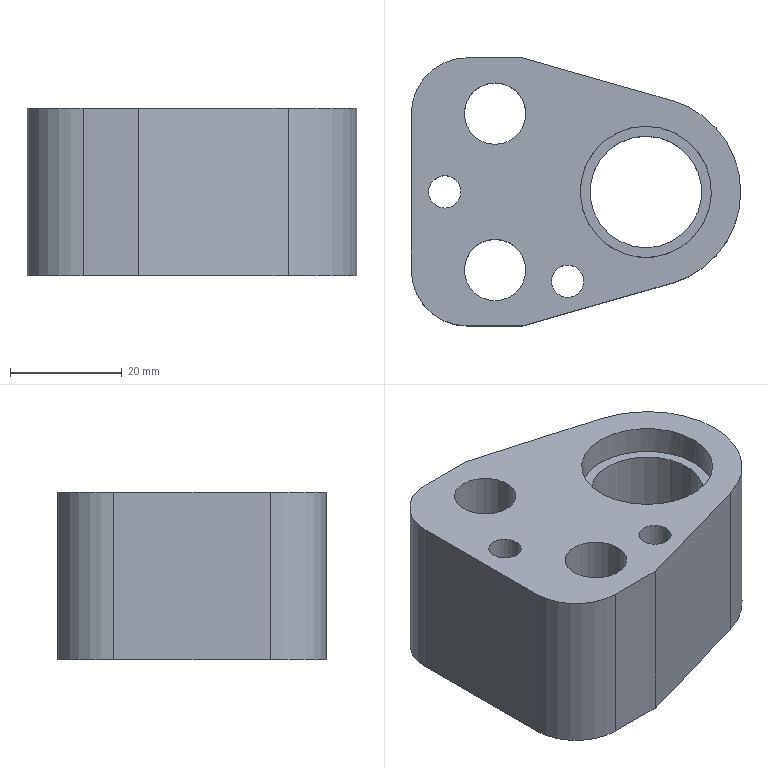Part | NX | features solid 2 | 1 solid | 25 faces | box 59 x 48 x 30 mm | volume 47279 mm3 | cylinder 13 | plane 12 | commonest cylinder face diameters 20 x3 5.8 x2 8 x2 11 x2 17 x2 23.5 x1
STEP:
#1=CARTESIAN_POINT('',(-406.,0.,201.));
#2=VERTEX_POINT('',#1);
#3=CARTESIAN_POINT('',(-379.31,7.66,201.));
#4=VERTEX_POINT('',#3);
#5=CARTESIAN_POINT('',(-386.776,5.517,201.));
#6=DIRECTION('',(0.9612,0.2759,0.));
#7=VECTOR('',#6,1000.);
#8=LINE('',#5,#7);
#9=EDGE_CURVE('',#2,#4,#8,.T.);
#10=ORIENTED_EDGE('',*,*,#9,.T.);
#11=CARTESIAN_POINT('',(-379.31,40.34,201.));
#12=VERTEX_POINT('',#11);
#13=CARTESIAN_POINT('',(-384.,24.,201.));
#14=DIRECTION('',(0.,0.,-1.));
#15=DIRECTION('',(0.,1.,0.));
#16=AXIS2_PLACEMENT_3D('',#13,#14,#15);
#17=CIRCLE('',#16,17.);
#18=EDGE_CURVE('',#12,#4,#17,.T.);
#19=ORIENTED_EDGE('',*,*,#18,.F.);
#20=CARTESIAN_POINT('',(-406.,48.,201.));
#21=VERTEX_POINT('',#20);
#22=CARTESIAN_POINT('',(-386.776,42.483,201.));
#23=DIRECTION('',(-0.9612,0.2759,0.));
#24=VECTOR('',#23,1000.);
#25=LINE('',#22,#24);
#26=EDGE_CURVE('',#12,#21,#25,.T.);
#27=ORIENTED_EDGE('',*,*,#26,.T.);
#28=CARTESIAN_POINT('',(-416.,48.,201.));
#29=VERTEX_POINT('',#28);
#30=CARTESIAN_POINT('',(-392.655,48.,201.));
#31=DIRECTION('',(1.,0.,0.));
#32=VECTOR('',#31,1000.);
#33=LINE('',#30,#32);
#34=EDGE_CURVE('',#29,#21,#33,.T.);
#35=ORIENTED_EDGE('',*,*,#34,.F.);
#36=CARTESIAN_POINT('',(-426.,38.,201.));
#37=VERTEX_POINT('',#36);
#38=CARTESIAN_POINT('',(-416.,38.,201.));
#39=DIRECTION('',(0.,0.,1.));
#40=DIRECTION('',(0.,-1.,0.));
#41=AXIS2_PLACEMENT_3D('',#38,#39,#40);
#42=CIRCLE('',#41,10.);
#43=EDGE_CURVE('',#29,#37,#42,.T.);
#44=ORIENTED_EDGE('',*,*,#43,.T.);
#45=CARTESIAN_POINT('',(-426.,10.,201.));
#46=VERTEX_POINT('',#45);
#47=CARTESIAN_POINT('',(-426.,24.,201.));
#48=DIRECTION('',(0.,1.,0.));
#49=VECTOR('',#48,1000.);
#50=LINE('',#47,#49);
#51=EDGE_CURVE('',#46,#37,#50,.T.);
#52=ORIENTED_EDGE('',*,*,#51,.F.);
#53=CARTESIAN_POINT('',(-416.,0.,201.));
#54=VERTEX_POINT('',#53);
#55=CARTESIAN_POINT('',(-416.,10.,201.));
#56=DIRECTION('',(0.,0.,1.));
#57=DIRECTION('',(0.,-1.,0.));
#58=AXIS2_PLACEMENT_3D('',#55,#56,#57);
#59=CIRCLE('',#58,10.);
#60=EDGE_CURVE('',#46,#54,#59,.T.);
#61=ORIENTED_EDGE('',*,*,#60,.T.);
#62=CARTESIAN_POINT('',(-392.655,0.,201.));
#63=DIRECTION('',(-1.,0.,0.));
#64=VECTOR('',#63,1000.);
#65=LINE('',#62,#64);
#66=EDGE_CURVE('',#2,#54,#65,.T.);
#67=ORIENTED_EDGE('',*,*,#66,.F.);
#68=EDGE_LOOP('',(#10,#19,#27,#35,#44,#52,#61,#67));
#69=FACE_BOUND('',#68,.T.);
#70=CARTESIAN_POINT('',(-420.,26.9,201.));
#71=VERTEX_POINT('',#70);
#72=CARTESIAN_POINT('',(-420.,24.,201.));
#73=DIRECTION('',(0.,0.,-1.));
#74=DIRECTION('',(0.,1.,0.));
#75=AXIS2_PLACEMENT_3D('',#72,#73,#74);
#76=CIRCLE('',#75,2.9);
#77=EDGE_CURVE('',#71,#71,#76,.T.);
#78=ORIENTED_EDGE('',*,*,#77,.T.);
#79=EDGE_LOOP('',(#78));
#80=FACE_BOUND('',#79,.T.);
#81=CARTESIAN_POINT('',(-398.,10.9,201.));
#82=VERTEX_POINT('',#81);
#83=CARTESIAN_POINT('',(-398.,8.,201.));
#84=DIRECTION('',(0.,0.,-1.));
#85=DIRECTION('',(0.,1.,0.));
#86=AXIS2_PLACEMENT_3D('',#83,#84,#85);
#87=CIRCLE('',#86,2.9);
#88=EDGE_CURVE('',#82,#82,#87,.T.);
#89=ORIENTED_EDGE('',*,*,#88,.T.);
#90=EDGE_LOOP('',(#89));
#91=FACE_BOUND('',#90,.T.);
#92=CARTESIAN_POINT('',(-411.,15.5,201.));
#93=VERTEX_POINT('',#92);
#94=CARTESIAN_POINT('',(-411.,10.,201.));
#95=DIRECTION('',(0.,0.,-1.));
#96=DIRECTION('',(0.,1.,0.));
#97=AXIS2_PLACEMENT_3D('',#94,#95,#96);
#98=CIRCLE('',#97,5.5);
#99=EDGE_CURVE('',#93,#93,#98,.T.);
#100=ORIENTED_EDGE('',*,*,#99,.T.);
#101=EDGE_LOOP('',(#100));
#102=FACE_BOUND('',#101,.T.);
#103=CARTESIAN_POINT('',(-411.,43.5,201.));
#104=VERTEX_POINT('',#103);
#105=CARTESIAN_POINT('',(-411.,38.,201.));
#106=DIRECTION('',(0.,0.,-1.));
#107=DIRECTION('',(0.,1.,0.));
#108=AXIS2_PLACEMENT_3D('',#105,#106,#107);
#109=CIRCLE('',#108,5.5);
#110=EDGE_CURVE('',#104,#104,#109,.T.);
#111=ORIENTED_EDGE('',*,*,#110,.T.);
#112=EDGE_LOOP('',(#111));
#113=FACE_BOUND('',#112,.T.);
#114=CARTESIAN_POINT('',(-384.,35.75,201.));
#115=VERTEX_POINT('',#114);
#116=CARTESIAN_POINT('',(-384.,24.,201.));
#117=DIRECTION('',(0.,0.,-1.));
#118=DIRECTION('',(0.,1.,0.));
#119=AXIS2_PLACEMENT_3D('',#116,#117,#118);
#120=CIRCLE('',#119,11.75);
#121=EDGE_CURVE('',#115,#115,#120,.T.);
#122=ORIENTED_EDGE('',*,*,#121,.T.);
#123=EDGE_LOOP('',(#122));
#124=FACE_BOUND('',#123,.T.);
#125=CARTESIAN_POINT('',(-392.655,24.,201.));
#126=DIRECTION('',(0.,0.,1.));
#127=DIRECTION('',(0.,-1.,0.));
#128=AXIS2_PLACEMENT_3D('',#125,#126,#127);
#129=PLANE('',#128);
#130=ADVANCED_FACE('',(#69,#80,#91,#102,#113,#124),#129,.T.);
#131=CARTESIAN_POINT('',(-406.,48.,171.));
#132=VERTEX_POINT('',#131);
#133=CARTESIAN_POINT('',(-406.,48.,171.));
#134=DIRECTION('',(0.,0.,1.));
#135=VECTOR('',#134,1000.);
#136=LINE('',#133,#135);
#137=EDGE_CURVE('',#132,#21,#136,.T.);
#138=ORIENTED_EDGE('',*,*,#137,.F.);
#139=CARTESIAN_POINT('',(-416.,48.,171.));
#140=VERTEX_POINT('',#139);
#141=CARTESIAN_POINT('',(-392.655,48.,171.));
#142=DIRECTION('',(-1.,0.,0.));
#143=VECTOR('',#142,1000.);
#144=LINE('',#141,#143);
#145=EDGE_CURVE('',#132,#140,#144,.T.);
#146=ORIENTED_EDGE('',*,*,#145,.T.);
#147=CARTESIAN_POINT('',(-416.,48.,171.));
#148=DIRECTION('',(0.,0.,1.));
#149=VECTOR('',#148,1000.);
#150=LINE('',#147,#149);
#151=EDGE_CURVE('',#140,#29,#150,.T.);
#152=ORIENTED_EDGE('',*,*,#151,.T.);
#153=ORIENTED_EDGE('',*,*,#34,.T.);
#154=EDGE_LOOP('',(#138,#146,#152,#153));
#155=FACE_BOUND('',#154,.T.);
#156=CARTESIAN_POINT('',(-392.655,48.,171.));
#157=DIRECTION('',(0.,1.,0.));
#158=DIRECTION('',(0.,0.,1.));
#159=AXIS2_PLACEMENT_3D('',#156,#157,#158);
#160=PLANE('',#159);
#161=ADVANCED_FACE('',(#155),#160,.T.);
#162=CARTESIAN_POINT('',(-379.31,7.66,171.));
#163=VERTEX_POINT('',#162);
#164=CARTESIAN_POINT('',(-406.,0.,171.));
#165=VERTEX_POINT('',#164);
#166=CARTESIAN_POINT('',(-386.776,5.517,171.));
#167=DIRECTION('',(-0.9612,-0.2759,0.));
#168=VECTOR('',#167,1000.);
#169=LINE('',#166,#168);
#170=EDGE_CURVE('',#163,#165,#169,.T.);
#171=ORIENTED_EDGE('',*,*,#170,.T.);
#172=CARTESIAN_POINT('',(-416.,0.,171.));
#173=VERTEX_POINT('',#172);
#174=CARTESIAN_POINT('',(-392.655,0.,171.));
#175=DIRECTION('',(1.,0.,0.));
#176=VECTOR('',#175,1000.);
#177=LINE('',#174,#176);
#178=EDGE_CURVE('',#173,#165,#177,.T.);
#179=ORIENTED_EDGE('',*,*,#178,.F.);
#180=CARTESIAN_POINT('',(-426.,10.,171.));
#181=VERTEX_POINT('',#180);
#182=CARTESIAN_POINT('',(-416.,10.,171.));
#183=DIRECTION('',(0.,0.,-1.));
#184=DIRECTION('',(0.,1.,0.));
#185=AXIS2_PLACEMENT_3D('',#182,#183,#184);
#186=CIRCLE('',#185,10.);
#187=EDGE_CURVE('',#173,#181,#186,.T.);
#188=ORIENTED_EDGE('',*,*,#187,.T.);
#189=CARTESIAN_POINT('',(-426.,38.,171.));
#190=VERTEX_POINT('',#189);
#191=CARTESIAN_POINT('',(-426.,24.,171.));
#192=DIRECTION('',(0.,-1.,0.));
#193=VECTOR('',#192,1000.);
#194=LINE('',#191,#193);
#195=EDGE_CURVE('',#190,#181,#194,.T.);
#196=ORIENTED_EDGE('',*,*,#195,.F.);
#197=CARTESIAN_POINT('',(-416.,38.,171.));
#198=DIRECTION('',(0.,0.,-1.));
#199=DIRECTION('',(0.,1.,0.));
#200=AXIS2_PLACEMENT_3D('',#197,#198,#199);
#201=CIRCLE('',#200,10.);
#202=EDGE_CURVE('',#190,#140,#201,.T.);
#203=ORIENTED_EDGE('',*,*,#202,.T.);
#204=ORIENTED_EDGE('',*,*,#145,.F.);
#205=CARTESIAN_POINT('',(-379.31,40.34,171.));
#206=VERTEX_POINT('',#205);
#207=CARTESIAN_POINT('',(-386.776,42.483,171.));
#208=DIRECTION('',(0.9612,-0.2759,0.));
#209=VECTOR('',#208,1000.);
#210=LINE('',#207,#209);
#211=EDGE_CURVE('',#132,#206,#210,.T.);
#212=ORIENTED_EDGE('',*,*,#211,.T.);
#213=CARTESIAN_POINT('',(-384.,24.,171.));
#214=DIRECTION('',(0.,0.,1.));
#215=DIRECTION('',(0.,-1.,0.));
#216=AXIS2_PLACEMENT_3D('',#213,#214,#215);
#217=CIRCLE('',#216,17.);
#218=EDGE_CURVE('',#163,#206,#217,.T.);
#219=ORIENTED_EDGE('',*,*,#218,.F.);
#220=EDGE_LOOP('',(#171,#179,#188,#196,#203,#204,#212,#219));
#221=FACE_BOUND('',#220,.T.);
#222=CARTESIAN_POINT('',(-420.,20.,171.));
#223=VERTEX_POINT('',#222);
#224=CARTESIAN_POINT('',(-420.,24.,171.));
#225=DIRECTION('',(0.,0.,1.));
#226=DIRECTION('',(0.,-1.,0.));
#227=AXIS2_PLACEMENT_3D('',#224,#225,#226);
#228=CIRCLE('',#227,4.);
#229=EDGE_CURVE('',#223,#223,#228,.T.);
#230=ORIENTED_EDGE('',*,*,#229,.T.);
#231=EDGE_LOOP('',(#230));
#232=FACE_BOUND('',#231,.T.);
#233=CARTESIAN_POINT('',(-398.,4.,171.));
#234=VERTEX_POINT('',#233);
#235=CARTESIAN_POINT('',(-398.,8.,171.));
#236=DIRECTION('',(0.,0.,1.));
#237=DIRECTION('',(0.,-1.,0.));
#238=AXIS2_PLACEMENT_3D('',#235,#236,#237);
#239=CIRCLE('',#238,4.);
#240=EDGE_CURVE('',#234,#234,#239,.T.);
#241=ORIENTED_EDGE('',*,*,#240,.T.);
#242=EDGE_LOOP('',(#241));
#243=FACE_BOUND('',#242,.T.);
#244=CARTESIAN_POINT('',(-411.,1.5,171.));
#245=VERTEX_POINT('',#244);
#246=CARTESIAN_POINT('',(-411.,10.,171.));
#247=DIRECTION('',(0.,0.,1.));
#248=DIRECTION('',(0.,-1.,0.));
#249=AXIS2_PLACEMENT_3D('',#246,#247,#248);
#250=CIRCLE('',#249,8.5);
#251=EDGE_CURVE('',#245,#245,#250,.T.);
#252=ORIENTED_EDGE('',*,*,#251,.T.);
#253=EDGE_LOOP('',(#252));
#254=FACE_BOUND('',#253,.T.);
#255=CARTESIAN_POINT('',(-411.,29.5,171.));
#256=VERTEX_POINT('',#255);
#257=CARTESIAN_POINT('',(-411.,38.,171.));
#258=DIRECTION('',(0.,0.,1.));
#259=DIRECTION('',(0.,-1.,0.));
#260=AXIS2_PLACEMENT_3D('',#257,#258,#259);
#261=CIRCLE('',#260,8.5);
#262=EDGE_CURVE('',#256,#256,#261,.T.);
#263=ORIENTED_EDGE('',*,*,#262,.T.);
#264=EDGE_LOOP('',(#263));
#265=FACE_BOUND('',#264,.T.);
#266=CARTESIAN_POINT('',(-384.,14.,171.));
#267=VERTEX_POINT('',#266);
#268=CARTESIAN_POINT('',(-384.,24.,171.));
#269=DIRECTION('',(0.,0.,1.));
#270=DIRECTION('',(0.,-1.,0.));
#271=AXIS2_PLACEMENT_3D('',#268,#269,#270);
#272=CIRCLE('',#271,10.);
#273=EDGE_CURVE('',#267,#267,#272,.T.);
#274=ORIENTED_EDGE('',*,*,#273,.T.);
#275=EDGE_LOOP('',(#274));
#276=FACE_BOUND('',#275,.T.);
#277=CARTESIAN_POINT('',(-392.655,24.,171.));
#278=DIRECTION('',(0.,0.,-1.));
#279=DIRECTION('',(0.,1.,0.));
#280=AXIS2_PLACEMENT_3D('',#277,#278,#279);
#281=PLANE('',#280);
#282=ADVANCED_FACE('',(#221,#232,#243,#254,#265,#276),#281,.T.);
#283=CARTESIAN_POINT('',(-406.,0.,171.));
#284=DIRECTION('',(0.,0.,1.));
#285=VECTOR('',#284,1000.);
#286=LINE('',#283,#285);
#287=EDGE_CURVE('',#165,#2,#286,.T.);
#288=ORIENTED_EDGE('',*,*,#287,.T.);
#289=ORIENTED_EDGE('',*,*,#66,.T.);
#290=CARTESIAN_POINT('',(-416.,0.,171.));
#291=DIRECTION('',(0.,0.,1.));
#292=VECTOR('',#291,1000.);
#293=LINE('',#290,#292);
#294=EDGE_CURVE('',#54,#173,#293,.F.);
#295=ORIENTED_EDGE('',*,*,#294,.T.);
#296=ORIENTED_EDGE('',*,*,#178,.T.);
#297=EDGE_LOOP('',(#288,#289,#295,#296));
#298=FACE_BOUND('',#297,.T.);
#299=CARTESIAN_POINT('',(-392.655,0.,171.));
#300=DIRECTION('',(0.,-1.,0.));
#301=DIRECTION('',(0.,0.,-1.));
#302=AXIS2_PLACEMENT_3D('',#299,#300,#301);
#303=PLANE('',#302);
#304=ADVANCED_FACE('',(#298),#303,.T.);
#305=ORIENTED_EDGE('',*,*,#18,.T.);
#306=CARTESIAN_POINT('',(-379.31,7.66,201.));
#307=DIRECTION('',(0.,0.,-1.));
#308=VECTOR('',#307,1000.);
#309=LINE('',#306,#308);
#310=EDGE_CURVE('',#4,#163,#309,.T.);
#311=ORIENTED_EDGE('',*,*,#310,.T.);
#312=ORIENTED_EDGE('',*,*,#218,.T.);
#313=CARTESIAN_POINT('',(-379.31,40.34,201.));
#314=DIRECTION('',(0.,0.,-1.));
#315=VECTOR('',#314,1000.);
#316=LINE('',#313,#315);
#317=EDGE_CURVE('',#206,#12,#316,.F.);
#318=ORIENTED_EDGE('',*,*,#317,.T.);
#319=EDGE_LOOP('',(#305,#311,#312,#318));
#320=FACE_BOUND('',#319,.T.);
#321=CARTESIAN_POINT('',(-384.,24.,201.));
#322=DIRECTION('',(0.,0.,-1.));
#323=DIRECTION('',(0.,1.,0.));
#324=AXIS2_PLACEMENT_3D('',#321,#322,#323);
#325=CYLINDRICAL_SURFACE('',#324,17.);
#326=ADVANCED_FACE('',(#320),#325,.T.);
#327=ORIENTED_EDGE('',*,*,#195,.T.);
#328=CARTESIAN_POINT('',(-426.,10.,171.));
#329=DIRECTION('',(0.,0.,1.));
#330=VECTOR('',#329,1000.);
#331=LINE('',#328,#330);
#332=EDGE_CURVE('',#181,#46,#331,.T.);
#333=ORIENTED_EDGE('',*,*,#332,.T.);
#334=ORIENTED_EDGE('',*,*,#51,.T.);
#335=CARTESIAN_POINT('',(-426.,38.,171.));
#336=DIRECTION('',(0.,0.,1.));
#337=VECTOR('',#336,1000.);
#338=LINE('',#335,#337);
#339=EDGE_CURVE('',#37,#190,#338,.F.);
#340=ORIENTED_EDGE('',*,*,#339,.T.);
#341=EDGE_LOOP('',(#327,#333,#334,#340));
#342=FACE_BOUND('',#341,.T.);
#343=CARTESIAN_POINT('',(-426.,24.,171.));
#344=DIRECTION('',(-1.,0.,0.));
#345=DIRECTION('',(0.,0.,-1.));
#346=AXIS2_PLACEMENT_3D('',#343,#344,#345);
#347=PLANE('',#346);
#348=ADVANCED_FACE('',(#342),#347,.T.);
#349=CARTESIAN_POINT('',(-384.,34.,196.));
#350=VERTEX_POINT('',#349);
#351=CARTESIAN_POINT('',(-384.,24.,196.));
#352=DIRECTION('',(0.,0.,-1.));
#353=DIRECTION('',(0.,1.,0.));
#354=AXIS2_PLACEMENT_3D('',#351,#352,#353);
#355=CIRCLE('',#354,10.);
#356=EDGE_CURVE('',#350,#350,#355,.T.);
#357=ORIENTED_EDGE('',*,*,#356,.T.);
#358=EDGE_LOOP('',(#357));
#359=FACE_BOUND('',#358,.T.);
#360=CARTESIAN_POINT('',(-384.,12.25,196.));
#361=VERTEX_POINT('',#360);
#362=CARTESIAN_POINT('',(-384.,24.,196.));
#363=DIRECTION('',(0.,0.,1.));
#364=DIRECTION('',(0.,-1.,0.));
#365=AXIS2_PLACEMENT_3D('',#362,#363,#364);
#366=CIRCLE('',#365,11.75);
#367=EDGE_CURVE('',#361,#361,#366,.T.);
#368=ORIENTED_EDGE('',*,*,#367,.T.);
#369=EDGE_LOOP('',(#368));
#370=FACE_BOUND('',#369,.T.);
#371=CARTESIAN_POINT('',(-384.,24.,196.));
#372=DIRECTION('',(0.,0.,-1.));
#373=DIRECTION('',(0.,1.,0.));
#374=AXIS2_PLACEMENT_3D('',#371,#372,#373);
#375=PLANE('',#374);
#376=ADVANCED_FACE('',(#359,#370),#375,.F.);
#377=ORIENTED_EDGE('',*,*,#367,.F.);
#378=EDGE_LOOP('',(#377));
#379=FACE_BOUND('',#378,.T.);
#380=ORIENTED_EDGE('',*,*,#121,.F.);
#381=EDGE_LOOP('',(#380));
#382=FACE_BOUND('',#381,.T.);
#383=CARTESIAN_POINT('',(-384.,24.,201.));
#384=DIRECTION('',(0.,0.,-1.));
#385=DIRECTION('',(0.,1.,0.));
#386=AXIS2_PLACEMENT_3D('',#383,#384,#385);
#387=CYLINDRICAL_SURFACE('',#386,11.75);
#388=ADVANCED_FACE('',(#379,#382),#387,.F.);
#389=ORIENTED_EDGE('',*,*,#273,.F.);
#390=EDGE_LOOP('',(#389));
#391=FACE_BOUND('',#390,.T.);
#392=ORIENTED_EDGE('',*,*,#356,.F.);
#393=EDGE_LOOP('',(#392));
#394=FACE_BOUND('',#393,.T.);
#395=CARTESIAN_POINT('',(-384.,24.,196.));
#396=DIRECTION('',(0.,0.,-1.));
#397=DIRECTION('',(0.,1.,0.));
#398=AXIS2_PLACEMENT_3D('',#395,#396,#397);
#399=CYLINDRICAL_SURFACE('',#398,10.);
#400=ADVANCED_FACE('',(#391,#394),#399,.F.);
#401=CARTESIAN_POINT('',(-411.,32.5,183.));
#402=VERTEX_POINT('',#401);
#403=CARTESIAN_POINT('',(-411.,38.,183.));
#404=DIRECTION('',(0.,0.,1.));
#405=DIRECTION('',(0.,-1.,0.));
#406=AXIS2_PLACEMENT_3D('',#403,#404,#405);
#407=CIRCLE('',#406,5.5);
#408=EDGE_CURVE('',#402,#402,#407,.F.);
#409=ORIENTED_EDGE('',*,*,#408,.T.);
#410=EDGE_LOOP('',(#409));
#411=FACE_BOUND('',#410,.T.);
#412=ORIENTED_EDGE('',*,*,#110,.F.);
#413=EDGE_LOOP('',(#412));
#414=FACE_BOUND('',#413,.T.);
#415=CARTESIAN_POINT('',(-411.,38.,201.));
#416=DIRECTION('',(0.,0.,-1.));
#417=DIRECTION('',(0.,1.,0.));
#418=AXIS2_PLACEMENT_3D('',#415,#416,#417);
#419=CYLINDRICAL_SURFACE('',#418,5.5);
#420=ADVANCED_FACE('',(#411,#414),#419,.F.);
#421=CARTESIAN_POINT('',(-411.,46.5,183.));
#422=VERTEX_POINT('',#421);
#423=CARTESIAN_POINT('',(-411.,38.,183.));
#424=DIRECTION('',(0.,0.,-1.));
#425=DIRECTION('',(0.,1.,0.));
#426=AXIS2_PLACEMENT_3D('',#423,#424,#425);
#427=CIRCLE('',#426,8.5);
#428=EDGE_CURVE('',#422,#422,#427,.T.);
#429=ORIENTED_EDGE('',*,*,#428,.T.);
#430=EDGE_LOOP('',(#429));
#431=FACE_BOUND('',#430,.T.);
#432=ORIENTED_EDGE('',*,*,#408,.F.);
#433=EDGE_LOOP('',(#432));
#434=FACE_BOUND('',#433,.T.);
#435=CARTESIAN_POINT('',(-411.,38.,183.));
#436=DIRECTION('',(0.,0.,1.));
#437=DIRECTION('',(0.,-1.,0.));
#438=AXIS2_PLACEMENT_3D('',#435,#436,#437);
#439=PLANE('',#438);
#440=ADVANCED_FACE('',(#431,#434),#439,.F.);
#441=ORIENTED_EDGE('',*,*,#262,.F.);
#442=EDGE_LOOP('',(#441));
#443=FACE_BOUND('',#442,.T.);
#444=ORIENTED_EDGE('',*,*,#428,.F.);
#445=EDGE_LOOP('',(#444));
#446=FACE_BOUND('',#445,.T.);
#447=CARTESIAN_POINT('',(-411.,38.,183.));
#448=DIRECTION('',(0.,0.,-1.));
#449=DIRECTION('',(0.,1.,0.));
#450=AXIS2_PLACEMENT_3D('',#447,#448,#449);
#451=CYLINDRICAL_SURFACE('',#450,8.5);
#452=ADVANCED_FACE('',(#443,#446),#451,.F.);
#453=CARTESIAN_POINT('',(-411.,4.5,183.));
#454=VERTEX_POINT('',#453);
#455=CARTESIAN_POINT('',(-411.,10.,183.));
#456=DIRECTION('',(0.,0.,1.));
#457=DIRECTION('',(0.,-1.,0.));
#458=AXIS2_PLACEMENT_3D('',#455,#456,#457);
#459=CIRCLE('',#458,5.5);
#460=EDGE_CURVE('',#454,#454,#459,.F.);
#461=ORIENTED_EDGE('',*,*,#460,.T.);
#462=EDGE_LOOP('',(#461));
#463=FACE_BOUND('',#462,.T.);
#464=ORIENTED_EDGE('',*,*,#99,.F.);
#465=EDGE_LOOP('',(#464));
#466=FACE_BOUND('',#465,.T.);
#467=CARTESIAN_POINT('',(-411.,10.,201.));
#468=DIRECTION('',(0.,0.,-1.));
#469=DIRECTION('',(0.,1.,0.));
#470=AXIS2_PLACEMENT_3D('',#467,#468,#469);
#471=CYLINDRICAL_SURFACE('',#470,5.5);
#472=ADVANCED_FACE('',(#463,#466),#471,.F.);
#473=CARTESIAN_POINT('',(-411.,18.5,183.));
#474=VERTEX_POINT('',#473);
#475=CARTESIAN_POINT('',(-411.,10.,183.));
#476=DIRECTION('',(0.,0.,-1.));
#477=DIRECTION('',(0.,1.,0.));
#478=AXIS2_PLACEMENT_3D('',#475,#476,#477);
#479=CIRCLE('',#478,8.5);
#480=EDGE_CURVE('',#474,#474,#479,.T.);
#481=ORIENTED_EDGE('',*,*,#480,.T.);
#482=EDGE_LOOP('',(#481));
#483=FACE_BOUND('',#482,.T.);
#484=ORIENTED_EDGE('',*,*,#460,.F.);
#485=EDGE_LOOP('',(#484));
#486=FACE_BOUND('',#485,.T.);
#487=CARTESIAN_POINT('',(-411.,10.,183.));
#488=DIRECTION('',(0.,0.,1.));
#489=DIRECTION('',(0.,-1.,0.));
#490=AXIS2_PLACEMENT_3D('',#487,#488,#489);
#491=PLANE('',#490);
#492=ADVANCED_FACE('',(#483,#486),#491,.F.);
#493=ORIENTED_EDGE('',*,*,#251,.F.);
#494=EDGE_LOOP('',(#493));
#495=FACE_BOUND('',#494,.T.);
#496=ORIENTED_EDGE('',*,*,#480,.F.);
#497=EDGE_LOOP('',(#496));
#498=FACE_BOUND('',#497,.T.);
#499=CARTESIAN_POINT('',(-411.,10.,183.));
#500=DIRECTION('',(0.,0.,-1.));
#501=DIRECTION('',(0.,1.,0.));
#502=AXIS2_PLACEMENT_3D('',#499,#500,#501);
#503=CYLINDRICAL_SURFACE('',#502,8.5);
#504=ADVANCED_FACE('',(#495,#498),#503,.F.);
#505=CARTESIAN_POINT('',(-398.,5.1,191.));
#506=VERTEX_POINT('',#505);
#507=CARTESIAN_POINT('',(-398.,8.,191.));
#508=DIRECTION('',(0.,0.,1.));
#509=DIRECTION('',(0.,-1.,0.));
#510=AXIS2_PLACEMENT_3D('',#507,#508,#509);
#511=CIRCLE('',#510,2.9);
#512=EDGE_CURVE('',#506,#506,#511,.F.);
#513=ORIENTED_EDGE('',*,*,#512,.T.);
#514=EDGE_LOOP('',(#513));
#515=FACE_BOUND('',#514,.T.);
#516=ORIENTED_EDGE('',*,*,#88,.F.);
#517=EDGE_LOOP('',(#516));
#518=FACE_BOUND('',#517,.T.);
#519=CARTESIAN_POINT('',(-398.,8.,201.));
#520=DIRECTION('',(0.,0.,-1.));
#521=DIRECTION('',(0.,1.,0.));
#522=AXIS2_PLACEMENT_3D('',#519,#520,#521);
#523=CYLINDRICAL_SURFACE('',#522,2.9);
#524=ADVANCED_FACE('',(#515,#518),#523,.F.);
#525=CARTESIAN_POINT('',(-398.,12.,191.));
#526=VERTEX_POINT('',#525);
#527=CARTESIAN_POINT('',(-398.,8.,191.));
#528=DIRECTION('',(0.,0.,-1.));
#529=DIRECTION('',(0.,1.,0.));
#530=AXIS2_PLACEMENT_3D('',#527,#528,#529);
#531=CIRCLE('',#530,4.);
#532=EDGE_CURVE('',#526,#526,#531,.T.);
#533=ORIENTED_EDGE('',*,*,#532,.T.);
#534=EDGE_LOOP('',(#533));
#535=FACE_BOUND('',#534,.T.);
#536=ORIENTED_EDGE('',*,*,#512,.F.);
#537=EDGE_LOOP('',(#536));
#538=FACE_BOUND('',#537,.T.);
#539=CARTESIAN_POINT('',(-398.,8.,191.));
#540=DIRECTION('',(0.,0.,1.));
#541=DIRECTION('',(0.,-1.,0.));
#542=AXIS2_PLACEMENT_3D('',#539,#540,#541);
#543=PLANE('',#542);
#544=ADVANCED_FACE('',(#535,#538),#543,.F.);
#545=ORIENTED_EDGE('',*,*,#240,.F.);
#546=EDGE_LOOP('',(#545));
#547=FACE_BOUND('',#546,.T.);
#548=ORIENTED_EDGE('',*,*,#532,.F.);
#549=EDGE_LOOP('',(#548));
#550=FACE_BOUND('',#549,.T.);
#551=CARTESIAN_POINT('',(-398.,8.,191.));
#552=DIRECTION('',(0.,0.,-1.));
#553=DIRECTION('',(0.,1.,0.));
#554=AXIS2_PLACEMENT_3D('',#551,#552,#553);
#555=CYLINDRICAL_SURFACE('',#554,4.);
#556=ADVANCED_FACE('',(#547,#550),#555,.F.);
#557=CARTESIAN_POINT('',(-420.,21.1,191.));
#558=VERTEX_POINT('',#557);
#559=CARTESIAN_POINT('',(-420.,24.,191.));
#560=DIRECTION('',(0.,0.,1.));
#561=DIRECTION('',(0.,-1.,0.));
#562=AXIS2_PLACEMENT_3D('',#559,#560,#561);
#563=CIRCLE('',#562,2.9);
#564=EDGE_CURVE('',#558,#558,#563,.F.);
#565=ORIENTED_EDGE('',*,*,#564,.T.);
#566=EDGE_LOOP('',(#565));
#567=FACE_BOUND('',#566,.T.);
#568=ORIENTED_EDGE('',*,*,#77,.F.);
#569=EDGE_LOOP('',(#568));
#570=FACE_BOUND('',#569,.T.);
#571=CARTESIAN_POINT('',(-420.,24.,201.));
#572=DIRECTION('',(0.,0.,-1.));
#573=DIRECTION('',(0.,1.,0.));
#574=AXIS2_PLACEMENT_3D('',#571,#572,#573);
#575=CYLINDRICAL_SURFACE('',#574,2.9);
#576=ADVANCED_FACE('',(#567,#570),#575,.F.);
#577=CARTESIAN_POINT('',(-420.,28.,191.));
#578=VERTEX_POINT('',#577);
#579=CARTESIAN_POINT('',(-420.,24.,191.));
#580=DIRECTION('',(0.,0.,-1.));
#581=DIRECTION('',(0.,1.,0.));
#582=AXIS2_PLACEMENT_3D('',#579,#580,#581);
#583=CIRCLE('',#582,4.);
#584=EDGE_CURVE('',#578,#578,#583,.T.);
#585=ORIENTED_EDGE('',*,*,#584,.T.);
#586=EDGE_LOOP('',(#585));
#587=FACE_BOUND('',#586,.T.);
#588=ORIENTED_EDGE('',*,*,#564,.F.);
#589=EDGE_LOOP('',(#588));
#590=FACE_BOUND('',#589,.T.);
#591=CARTESIAN_POINT('',(-420.,24.,191.));
#592=DIRECTION('',(0.,0.,1.));
#593=DIRECTION('',(0.,-1.,0.));
#594=AXIS2_PLACEMENT_3D('',#591,#592,#593);
#595=PLANE('',#594);
#596=ADVANCED_FACE('',(#587,#590),#595,.F.);
#597=ORIENTED_EDGE('',*,*,#229,.F.);
#598=EDGE_LOOP('',(#597));
#599=FACE_BOUND('',#598,.T.);
#600=ORIENTED_EDGE('',*,*,#584,.F.);
#601=EDGE_LOOP('',(#600));
#602=FACE_BOUND('',#601,.T.);
#603=CARTESIAN_POINT('',(-420.,24.,191.));
#604=DIRECTION('',(0.,0.,-1.));
#605=DIRECTION('',(0.,1.,0.));
#606=AXIS2_PLACEMENT_3D('',#603,#604,#605);
#607=CYLINDRICAL_SURFACE('',#606,4.);
#608=ADVANCED_FACE('',(#599,#602),#607,.F.);
#609=ORIENTED_EDGE('',*,*,#187,.F.);
#610=ORIENTED_EDGE('',*,*,#294,.F.);
#611=ORIENTED_EDGE('',*,*,#60,.F.);
#612=ORIENTED_EDGE('',*,*,#332,.F.);
#613=EDGE_LOOP('',(#609,#610,#611,#612));
#614=FACE_BOUND('',#613,.T.);
#615=CARTESIAN_POINT('',(-416.,10.,171.));
#616=DIRECTION('',(0.,0.,1.));
#617=DIRECTION('',(0.,-1.,0.));
#618=AXIS2_PLACEMENT_3D('',#615,#616,#617);
#619=CYLINDRICAL_SURFACE('',#618,10.);
#620=ADVANCED_FACE('',(#614),#619,.T.);
#621=ORIENTED_EDGE('',*,*,#202,.F.);
#622=ORIENTED_EDGE('',*,*,#339,.F.);
#623=ORIENTED_EDGE('',*,*,#43,.F.);
#624=ORIENTED_EDGE('',*,*,#151,.F.);
#625=EDGE_LOOP('',(#621,#622,#623,#624));
#626=FACE_BOUND('',#625,.T.);
#627=CARTESIAN_POINT('',(-416.,38.,171.));
#628=DIRECTION('',(0.,0.,1.));
#629=DIRECTION('',(0.,-1.,0.));
#630=AXIS2_PLACEMENT_3D('',#627,#628,#629);
#631=CYLINDRICAL_SURFACE('',#630,10.);
#632=ADVANCED_FACE('',(#626),#631,.T.);
#633=ORIENTED_EDGE('',*,*,#317,.F.);
#634=ORIENTED_EDGE('',*,*,#211,.F.);
#635=ORIENTED_EDGE('',*,*,#137,.T.);
#636=ORIENTED_EDGE('',*,*,#26,.F.);
#637=EDGE_LOOP('',(#633,#634,#635,#636));
#638=FACE_BOUND('',#637,.T.);
#639=CARTESIAN_POINT('',(-386.776,42.483,171.));
#640=DIRECTION('',(-0.2759,-0.9612,0.));
#641=DIRECTION('',(0.,0.,-1.));
#642=AXIS2_PLACEMENT_3D('',#639,#640,#641);
#643=PLANE('',#642);
#644=ADVANCED_FACE('',(#638),#643,.F.);
#645=ORIENTED_EDGE('',*,*,#310,.F.);
#646=ORIENTED_EDGE('',*,*,#9,.F.);
#647=ORIENTED_EDGE('',*,*,#287,.F.);
#648=ORIENTED_EDGE('',*,*,#170,.F.);
#649=EDGE_LOOP('',(#645,#646,#647,#648));
#650=FACE_BOUND('',#649,.T.);
#651=CARTESIAN_POINT('',(-386.776,5.517,171.));
#652=DIRECTION('',(-0.2759,0.9612,0.));
#653=DIRECTION('',(0.,0.,1.));
#654=AXIS2_PLACEMENT_3D('',#651,#652,#653);
#655=PLANE('',#654);
#656=ADVANCED_FACE('',(#650),#655,.F.);
#657=CLOSED_SHELL('',(#130,#161,#282,#304,#326,#348,#376,#388,#400,#420,#440,#452,#472,#492,#504,#524,#544,#556,#576,#596,#608,#620,#632,#644,#656));
#658=MANIFOLD_SOLID_BREP('',#657);
#659=(LENGTH_UNIT()NAMED_UNIT(*)SI_UNIT(.MILLI.,.METRE.));
#660=UNCERTAINTY_MEASURE_WITH_UNIT(LENGTH_MEASURE(0.00001),#659,'','');
#661=(NAMED_UNIT(*)PLANE_ANGLE_UNIT()SI_UNIT($,.RADIAN.));
#662=(NAMED_UNIT(*)SI_UNIT($,.STERADIAN.)SOLID_ANGLE_UNIT());
#663=(GEOMETRIC_REPRESENTATION_CONTEXT(3)GLOBAL_UNCERTAINTY_ASSIGNED_CONTEXT((#660))GLOBAL_UNIT_ASSIGNED_CONTEXT((#659,#661,#662))REPRESENTATION_CONTEXT('',''));
#664=ADVANCED_BREP_SHAPE_REPRESENTATION('',(#658),#663);